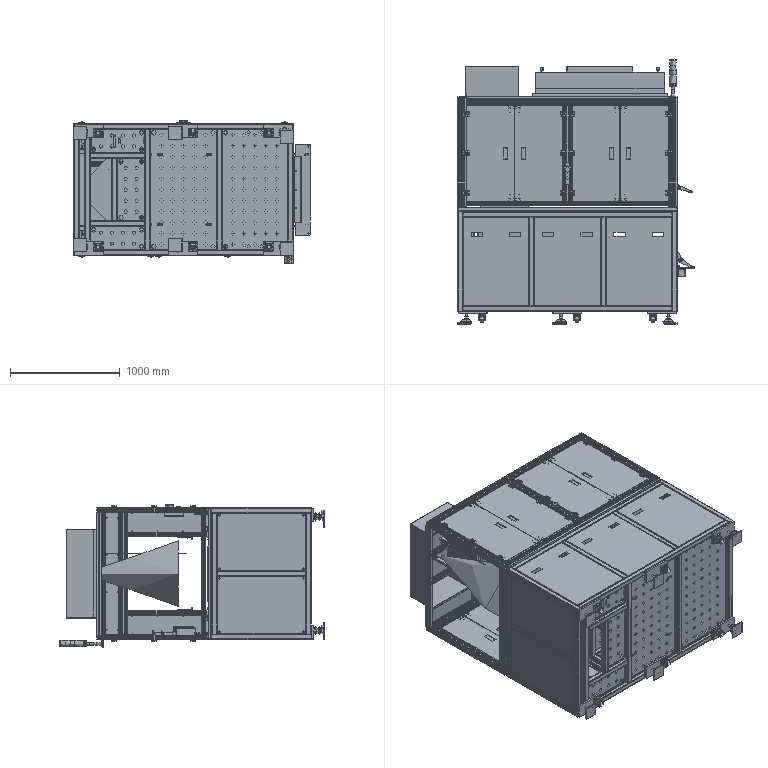Part | NX | 440 solids | 17756 faces | volume 422706573 mm3 | plane 11354 | cylinder 4934 | cone 726 | spline 627 | torus 90 | sphere 25 | commonest cylinder face diameters 4 x443 6 x294 8 x235 30 x218 14 x198 2 x195